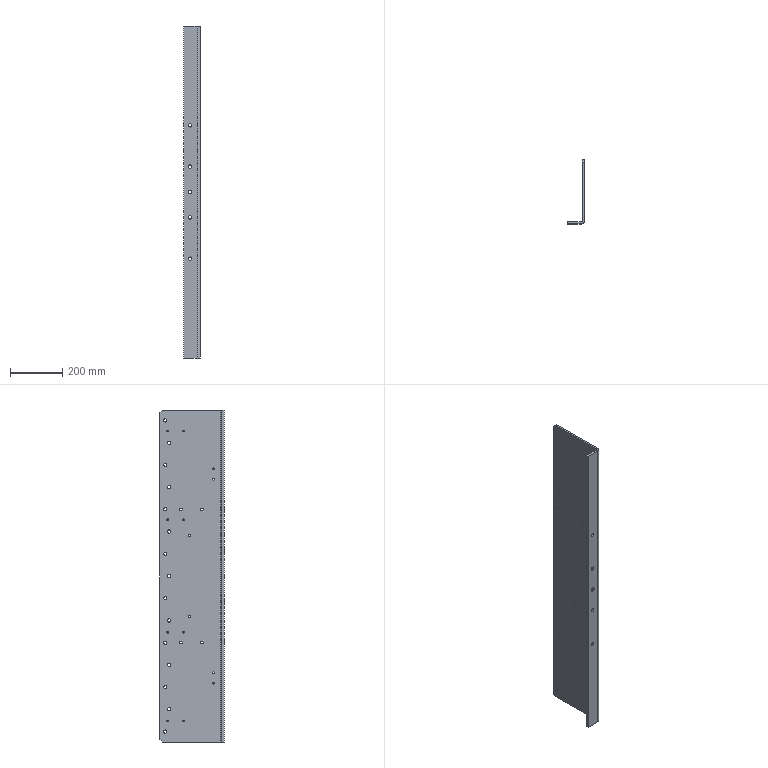Part | SolidWorks | features ICE 4, HoleWzd 2, Chamfer 1, Extrusion 1 | 1 solid | 118 faces | box 65 x 245 x 1270 mm | volume 2991073 mm3 | cylinder 78 | cone 30 | plane 10 | commonest cylinder face diameters 12.5 x30 6.8 x24 10.2 x8 13 x8 10.5 x4 15 x2